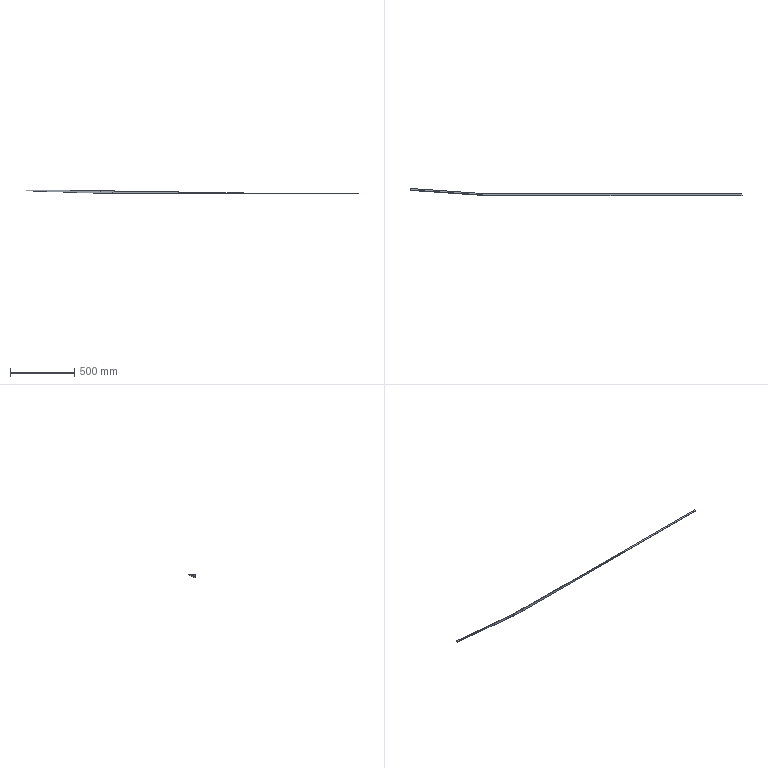Part | SolidWorks | features BaseBody 1 | 1 solid | 18 faces | box 2582 x 55.311 x 25.611 mm | volume 177639 mm3 | plane 18
STEP:
#1=CARTESIAN_POINT('',(2000.,-23.156,0.4292));
#2=VERTEX_POINT('',#1);
#3=CARTESIAN_POINT('',(90.138,-23.157,0.4297));
#4=VERTEX_POINT('',#3);
#5=CARTESIAN_POINT('',(2000.,-23.156,0.4292));
#6=DIRECTION('',(-1.,-0.00000047,0.000000257));
#7=VECTOR('',#6,1000.);
#8=LINE('',#5,#7);
#9=EDGE_CURVE('',#2,#4,#8,.T.);
#10=ORIENTED_EDGE('',*,*,#9,.T.);
#11=CARTESIAN_POINT('',(90.189,-23.22,3.629));
#12=VERTEX_POINT('',#11);
#13=CARTESIAN_POINT('',(90.138,-23.157,0.4297));
#14=DIRECTION('',(0.01588,-0.01967,0.9997));
#15=VECTOR('',#14,1000.);
#16=LINE('',#13,#15);
#17=EDGE_CURVE('',#4,#12,#16,.T.);
#18=ORIENTED_EDGE('',*,*,#17,.T.);
#19=CARTESIAN_POINT('',(2000.,-23.219,3.629));
#20=VERTEX_POINT('',#19);
#21=CARTESIAN_POINT('',(90.189,-23.22,3.629));
#22=DIRECTION('',(1.,0.00000047,-0.000000257));
#23=VECTOR('',#22,1000.);
#24=LINE('',#21,#23);
#25=EDGE_CURVE('',#12,#20,#24,.T.);
#26=ORIENTED_EDGE('',*,*,#25,.T.);
#27=CARTESIAN_POINT('',(2000.,-23.188,2.029));
#28=DIRECTION('',(0.,0.01967,-0.9998));
#29=VECTOR('',#28,1000.);
#30=LINE('',#27,#29);
#31=EDGE_CURVE('',#20,#2,#30,.T.);
#32=ORIENTED_EDGE('',*,*,#31,.T.);
#33=EDGE_LOOP('',(#10,#18,#26,#32));
#34=FACE_OUTER_BOUND('',#33,.T.);
#35=CARTESIAN_POINT('',(78.679,-23.157,0.41));
#36=DIRECTION('',(-0.000000465,0.9998,0.01967));
#37=DIRECTION('',(0.,-0.01967,0.9998));
#38=AXIS2_PLACEMENT_3D('',#35,#36,#37);
#39=PLANE('',#38);
#40=ADVANCED_FACE('',(#34),#39,.T.);
#41=CARTESIAN_POINT('',(-5.976,-23.214,3.483));
#42=VERTEX_POINT('',#41);
#43=CARTESIAN_POINT('',(-5.976,-23.214,3.483));
#44=DIRECTION('',(0.9995,0.0005894,-0.03175));
#45=VECTOR('',#44,1000.);
#46=LINE('',#43,#45);
#47=EDGE_CURVE('',#42,#4,#46,.T.);
#48=ORIENTED_EDGE('',*,*,#47,.F.);
#49=CARTESIAN_POINT('',(-5.875,-23.277,6.68));
#50=VERTEX_POINT('',#49);
#51=CARTESIAN_POINT('',(-5.875,-23.277,6.68));
#52=DIRECTION('',(-0.03175,0.01966,-0.9993));
#53=VECTOR('',#52,1000.);
#54=LINE('',#51,#53);
#55=EDGE_CURVE('',#50,#42,#54,.T.);
#56=ORIENTED_EDGE('',*,*,#55,.F.);
#57=CARTESIAN_POINT('',(90.189,-23.22,3.629));
#58=DIRECTION('',(-0.9995,-0.0005894,0.03175));
#59=VECTOR('',#58,1000.);
#60=LINE('',#57,#59);
#61=EDGE_CURVE('',#12,#50,#60,.T.);
#62=ORIENTED_EDGE('',*,*,#61,.F.);
#63=ORIENTED_EDGE('',*,*,#17,.F.);
#64=EDGE_LOOP('',(#48,#56,#62,#63));
#65=FACE_OUTER_BOUND('',#64,.T.);
#66=CARTESIAN_POINT('',(-6.553,-23.278,6.718));
#67=DIRECTION('',(-0.00003526,-0.9998,-0.01967));
#68=DIRECTION('',(0.,0.01967,-0.9998));
#69=AXIS2_PLACEMENT_3D('',#66,#67,#68);
#70=PLANE('',#69);
#71=ADVANCED_FACE('',(#65),#70,.F.);
#72=CARTESIAN_POINT('',(2000.,-38.156,0.1341));
#73=VERTEX_POINT('',#72);
#74=CARTESIAN_POINT('',(90.138,-38.157,0.1346));
#75=VERTEX_POINT('',#74);
#76=CARTESIAN_POINT('',(2000.,-38.156,0.1341));
#77=DIRECTION('',(-1.,-0.00000047,0.000000257));
#78=VECTOR('',#77,1000.);
#79=LINE('',#76,#78);
#80=EDGE_CURVE('',#73,#75,#79,.T.);
#81=ORIENTED_EDGE('',*,*,#80,.T.);
#82=CARTESIAN_POINT('',(90.138,-38.157,0.1346));
#83=DIRECTION('',(0.00001742,0.9998,0.01967));
#84=VECTOR('',#83,1000.);
#85=LINE('',#82,#84);
#86=EDGE_CURVE('',#75,#4,#85,.T.);
#87=ORIENTED_EDGE('',*,*,#86,.T.);
#88=ORIENTED_EDGE('',*,*,#9,.F.);
#89=CARTESIAN_POINT('',(2000.,-38.247,0.1323));
#90=DIRECTION('',(0.,-0.9998,-0.01967));
#91=VECTOR('',#90,1000.);
#92=LINE('',#89,#91);
#93=EDGE_CURVE('',#2,#73,#92,.T.);
#94=ORIENTED_EDGE('',*,*,#93,.T.);
#95=EDGE_LOOP('',(#81,#87,#88,#94));
#96=FACE_OUTER_BOUND('',#95,.T.);
#97=CARTESIAN_POINT('',(78.679,-38.247,0.1328));
#98=DIRECTION('',(-0.000000266,0.01967,-0.9998));
#99=DIRECTION('',(0.,0.9998,0.01967));
#100=AXIS2_PLACEMENT_3D('',#97,#98,#99);
#101=PLANE('',#100);
#102=ADVANCED_FACE('',(#96),#101,.T.);
#103=ORIENTED_EDGE('',*,*,#93,.F.);
#104=ORIENTED_EDGE('',*,*,#31,.F.);
#105=CARTESIAN_POINT('',(2000.,-38.219,3.333));
#106=VERTEX_POINT('',#105);
#107=CARTESIAN_POINT('',(2000.,-23.219,3.629));
#108=DIRECTION('',(0.000000465,-0.9998,-0.01967));
#109=VECTOR('',#108,1000.);
#110=LINE('',#107,#109);
#111=EDGE_CURVE('',#20,#106,#110,.T.);
#112=ORIENTED_EDGE('',*,*,#111,.T.);
#113=CARTESIAN_POINT('',(2000.,-38.219,3.333));
#114=DIRECTION('',(-0.000000266,0.01967,-0.9998));
#115=VECTOR('',#114,1000.);
#116=LINE('',#113,#115);
#117=EDGE_CURVE('',#106,#73,#116,.T.);
#118=ORIENTED_EDGE('',*,*,#117,.T.);
#119=EDGE_LOOP('',(#103,#104,#112,#118));
#120=FACE_OUTER_BOUND('',#119,.T.);
#121=CARTESIAN_POINT('',(2000.,-38.309,0.1131));
#122=DIRECTION('',(1.,0.00000047,-0.000000257));
#123=DIRECTION('',(-0.00000047,1.,0.));
#124=AXIS2_PLACEMENT_3D('',#121,#122,#123);
#125=PLANE('',#124);
#126=ADVANCED_FACE('',(#120),#125,.T.);
#127=ORIENTED_EDGE('',*,*,#25,.F.);
#128=CARTESIAN_POINT('',(90.189,-35.02,3.397));
#129=VERTEX_POINT('',#128);
#130=CARTESIAN_POINT('',(90.189,-23.22,3.629));
#131=DIRECTION('',(-0.00001748,-0.9998,-0.01967));
#132=VECTOR('',#131,1000.);
#133=LINE('',#130,#132);
#134=EDGE_CURVE('',#12,#129,#133,.T.);
#135=ORIENTED_EDGE('',*,*,#134,.T.);
#136=CARTESIAN_POINT('',(1223.273,-35.02,3.397));
#137=VERTEX_POINT('',#136);
#138=CARTESIAN_POINT('',(90.189,-35.02,3.397));
#139=DIRECTION('',(1.,0.00000047,-0.000000257));
#140=VECTOR('',#139,1000.);
#141=LINE('',#138,#140);
#142=EDGE_CURVE('',#129,#137,#141,.T.);
#143=ORIENTED_EDGE('',*,*,#142,.T.);
#144=CARTESIAN_POINT('',(1223.273,-38.219,3.334));
#145=VERTEX_POINT('',#144);
#146=CARTESIAN_POINT('',(1223.273,-30.719,3.481));
#147=DIRECTION('',(0.,-0.9998,-0.01967));
#148=VECTOR('',#147,1000.);
#149=LINE('',#146,#148);
#150=EDGE_CURVE('',#137,#145,#149,.T.);
#151=ORIENTED_EDGE('',*,*,#150,.T.);
#152=CARTESIAN_POINT('',(1223.273,-38.219,3.334));
#153=DIRECTION('',(1.,0.00000047,-0.000000257));
#154=VECTOR('',#153,1000.);
#155=LINE('',#152,#154);
#156=EDGE_CURVE('',#145,#106,#155,.T.);
#157=ORIENTED_EDGE('',*,*,#156,.T.);
#158=ORIENTED_EDGE('',*,*,#111,.F.);
#159=EDGE_LOOP('',(#127,#135,#143,#151,#157,#158));
#160=FACE_OUTER_BOUND('',#159,.T.);
#161=CARTESIAN_POINT('',(90.189,-23.219,3.629));
#162=DIRECTION('',(0.000000266,-0.01967,0.9998));
#163=DIRECTION('',(0.,-0.9998,-0.01967));
#164=AXIS2_PLACEMENT_3D('',#161,#162,#163);
#165=PLANE('',#164);
#166=ADVANCED_FACE('',(#160),#165,.T.);
#167=CARTESIAN_POINT('',(-6.5,-38.214,3.204));
#168=VERTEX_POINT('',#167);
#169=CARTESIAN_POINT('',(-582.328,1.725,22.286));
#170=VERTEX_POINT('',#169);
#171=CARTESIAN_POINT('',(-6.5,-38.214,3.204));
#172=DIRECTION('',(-0.9971,0.06916,0.03304));
#173=VECTOR('',#172,1000.);
#174=LINE('',#171,#173);
#175=EDGE_CURVE('',#168,#170,#174,.T.);
#176=ORIENTED_EDGE('',*,*,#175,.T.);
#177=CARTESIAN_POINT('',(-581.281,16.689,22.548));
#178=VERTEX_POINT('',#177);
#179=CARTESIAN_POINT('',(-582.328,1.725,22.286));
#180=DIRECTION('',(0.06976,0.9974,0.01741));
#181=VECTOR('',#180,1000.);
#182=LINE('',#179,#181);
#183=EDGE_CURVE('',#170,#178,#182,.T.);
#184=ORIENTED_EDGE('',*,*,#183,.T.);
#185=CARTESIAN_POINT('',(-581.281,16.689,22.548));
#186=DIRECTION('',(0.9971,-0.06916,-0.03304));
#187=VECTOR('',#186,1000.);
#188=LINE('',#185,#187);
#189=EDGE_CURVE('',#178,#42,#188,.T.);
#190=ORIENTED_EDGE('',*,*,#189,.T.);
#191=ORIENTED_EDGE('',*,*,#47,.T.);
#192=ORIENTED_EDGE('',*,*,#86,.F.);
#193=CARTESIAN_POINT('',(90.138,-38.157,0.1346));
#194=DIRECTION('',(-0.9995,-0.0005894,0.03175));
#195=VECTOR('',#194,1000.);
#196=LINE('',#193,#195);
#197=EDGE_CURVE('',#75,#168,#196,.T.);
#198=ORIENTED_EDGE('',*,*,#197,.T.);
#199=EDGE_LOOP('',(#176,#184,#190,#191,#192,#198));
#200=FACE_OUTER_BOUND('',#199,.T.);
#201=CARTESIAN_POINT('',(90.138,-38.214,0.1335));
#202=DIRECTION('',(-0.03175,0.01966,-0.9993));
#203=DIRECTION('',(-0.9995,0.,0.03176));
#204=AXIS2_PLACEMENT_3D('',#201,#202,#203);
#205=PLANE('',#204);
#206=ADVANCED_FACE('',(#200),#205,.T.);
#207=ORIENTED_EDGE('',*,*,#189,.F.);
#208=CARTESIAN_POINT('',(-581.18,16.626,25.745));
#209=VERTEX_POINT('',#208);
#210=CARTESIAN_POINT('',(-581.281,16.689,22.548));
#211=DIRECTION('',(0.03175,-0.01966,0.9993));
#212=VECTOR('',#211,1000.);
#213=LINE('',#210,#212);
#214=EDGE_CURVE('',#178,#209,#213,.T.);
#215=ORIENTED_EDGE('',*,*,#214,.T.);
#216=CARTESIAN_POINT('',(-581.18,16.626,25.745));
#217=DIRECTION('',(0.9971,-0.06916,-0.03304));
#218=VECTOR('',#217,1000.);
#219=LINE('',#216,#218);
#220=EDGE_CURVE('',#209,#50,#219,.T.);
#221=ORIENTED_EDGE('',*,*,#220,.T.);
#222=ORIENTED_EDGE('',*,*,#55,.T.);
#223=EDGE_LOOP('',(#207,#215,#221,#222));
#224=FACE_OUTER_BOUND('',#223,.T.);
#225=CARTESIAN_POINT('',(-2.418,-23.46,3.349));
#226=DIRECTION('',(0.06976,0.9974,0.01741));
#227=DIRECTION('',(-0.9976,0.06977,0.));
#228=AXIS2_PLACEMENT_3D('',#225,#226,#227);
#229=PLANE('',#228);
#230=ADVANCED_FACE('',(#224),#229,.T.);
#231=ORIENTED_EDGE('',*,*,#220,.F.);
#232=CARTESIAN_POINT('',(-582.003,4.854,25.54));
#233=VERTEX_POINT('',#232);
#234=CARTESIAN_POINT('',(-581.18,16.626,25.745));
#235=DIRECTION('',(-0.06976,-0.9974,-0.01741));
#236=VECTOR('',#235,1000.);
#237=LINE('',#234,#236);
#238=EDGE_CURVE('',#209,#233,#237,.T.);
#239=ORIENTED_EDGE('',*,*,#238,.T.);
#240=CARTESIAN_POINT('',(-6.287,-35.077,6.461));
#241=VERTEX_POINT('',#240);
#242=CARTESIAN_POINT('',(-582.003,4.854,25.54));
#243=DIRECTION('',(0.9971,-0.06916,-0.03304));
#244=VECTOR('',#243,1000.);
#245=LINE('',#242,#244);
#246=EDGE_CURVE('',#233,#241,#245,.T.);
#247=ORIENTED_EDGE('',*,*,#246,.T.);
#248=CARTESIAN_POINT('',(-6.287,-35.077,6.461));
#249=DIRECTION('',(0.9995,0.0005894,-0.03175));
#250=VECTOR('',#249,1000.);
#251=LINE('',#248,#250);
#252=EDGE_CURVE('',#241,#129,#251,.T.);
#253=ORIENTED_EDGE('',*,*,#252,.T.);
#254=ORIENTED_EDGE('',*,*,#134,.F.);
#255=ORIENTED_EDGE('',*,*,#61,.T.);
#256=EDGE_LOOP('',(#231,#239,#247,#253,#254,#255));
#257=FACE_OUTER_BOUND('',#256,.T.);
#258=CARTESIAN_POINT('',(-582.028,-35.077,24.755));
#259=DIRECTION('',(0.03175,-0.01966,0.9993));
#260=DIRECTION('',(0.9995,0.,-0.03176));
#261=AXIS2_PLACEMENT_3D('',#258,#259,#260);
#262=PLANE('',#261);
#263=ADVANCED_FACE('',(#257),#262,.T.);
#264=ORIENTED_EDGE('',*,*,#80,.F.);
#265=ORIENTED_EDGE('',*,*,#117,.F.);
#266=ORIENTED_EDGE('',*,*,#156,.F.);
#267=CARTESIAN_POINT('',(90.468,-38.566,20.934));
#268=VERTEX_POINT('',#267);
#269=CARTESIAN_POINT('',(1223.273,-38.219,3.334));
#270=DIRECTION('',(-0.9999,-0.0003061,0.01553));
#271=VECTOR('',#270,1000.);
#272=LINE('',#269,#271);
#273=EDGE_CURVE('',#145,#268,#272,.T.);
#274=ORIENTED_EDGE('',*,*,#273,.T.);
#275=CARTESIAN_POINT('',(90.468,-38.566,20.934));
#276=DIRECTION('',(-0.01588,0.01967,-0.9997));
#277=VECTOR('',#276,1000.);
#278=LINE('',#275,#277);
#279=EDGE_CURVE('',#268,#75,#278,.T.);
#280=ORIENTED_EDGE('',*,*,#279,.T.);
#281=EDGE_LOOP('',(#264,#265,#266,#274,#280));
#282=FACE_OUTER_BOUND('',#281,.T.);
#283=CARTESIAN_POINT('',(90.138,-38.566,20.934));
#284=DIRECTION('',(0.000000465,-0.9998,-0.01967));
#285=DIRECTION('',(0.,0.01967,-0.9998));
#286=AXIS2_PLACEMENT_3D('',#283,#284,#285);
#287=PLANE('',#286);
#288=ADVANCED_FACE('',(#282),#287,.T.);
#289=ORIENTED_EDGE('',*,*,#150,.F.);
#290=CARTESIAN_POINT('',(90.468,-35.367,20.997));
#291=VERTEX_POINT('',#290);
#292=CARTESIAN_POINT('',(90.468,-35.367,20.997));
#293=DIRECTION('',(0.9999,0.0003061,-0.01553));
#294=VECTOR('',#293,1000.);
#295=LINE('',#292,#294);
#296=EDGE_CURVE('',#291,#137,#295,.T.);
#297=ORIENTED_EDGE('',*,*,#296,.F.);
#298=CARTESIAN_POINT('',(90.468,-38.566,20.934));
#299=DIRECTION('',(0.00003449,0.9998,0.01967));
#300=VECTOR('',#299,1000.);
#301=LINE('',#298,#300);
#302=EDGE_CURVE('',#268,#291,#301,.T.);
#303=ORIENTED_EDGE('',*,*,#302,.F.);
#304=ORIENTED_EDGE('',*,*,#273,.F.);
#305=EDGE_LOOP('',(#289,#297,#303,#304));
#306=FACE_OUTER_BOUND('',#305,.T.);
#307=CARTESIAN_POINT('',(90.468,-38.585,20.933));
#308=DIRECTION('',(-0.01554,0.01967,-0.9997));
#309=DIRECTION('',(0.,0.9998,0.01967));
#310=AXIS2_PLACEMENT_3D('',#307,#308,#309);
#311=PLANE('',#310);
#312=ADVANCED_FACE('',(#306),#311,.F.);
#313=ORIENTED_EDGE('',*,*,#142,.F.);
#314=CARTESIAN_POINT('',(90.189,-35.02,3.397));
#315=DIRECTION('',(0.01588,-0.01967,0.9997));
#316=VECTOR('',#315,1000.);
#317=LINE('',#314,#316);
#318=EDGE_CURVE('',#129,#291,#317,.T.);
#319=ORIENTED_EDGE('',*,*,#318,.T.);
#320=ORIENTED_EDGE('',*,*,#296,.T.);
#321=EDGE_LOOP('',(#313,#319,#320));
#322=FACE_OUTER_BOUND('',#321,.T.);
#323=CARTESIAN_POINT('',(83.39,-35.018,3.291));
#324=DIRECTION('',(-0.000000465,0.9998,0.01967));
#325=DIRECTION('',(0.,-0.01967,0.9998));
#326=AXIS2_PLACEMENT_3D('',#323,#324,#325);
#327=PLANE('',#326);
#328=ADVANCED_FACE('',(#322),#327,.T.);
#329=CARTESIAN_POINT('',(-582.226,1.662,25.484));
#330=VERTEX_POINT('',#329);
#331=CARTESIAN_POINT('',(-582.003,4.854,25.54));
#332=DIRECTION('',(-0.06976,-0.9974,-0.01741));
#333=VECTOR('',#332,1000.);
#334=LINE('',#331,#333);
#335=EDGE_CURVE('',#233,#330,#334,.T.);
#336=ORIENTED_EDGE('',*,*,#335,.F.);
#337=ORIENTED_EDGE('',*,*,#238,.F.);
#338=ORIENTED_EDGE('',*,*,#214,.F.);
#339=ORIENTED_EDGE('',*,*,#183,.F.);
#340=CARTESIAN_POINT('',(-582.226,1.662,25.484));
#341=DIRECTION('',(-0.03175,0.01966,-0.9993));
#342=VECTOR('',#341,1000.);
#343=LINE('',#340,#342);
#344=EDGE_CURVE('',#330,#170,#343,.T.);
#345=ORIENTED_EDGE('',*,*,#344,.F.);
#346=EDGE_LOOP('',(#336,#337,#338,#339,#345));
#347=FACE_OUTER_BOUND('',#346,.T.);
#348=CARTESIAN_POINT('',(-582.332,1.67,22.286));
#349=DIRECTION('',(0.9971,-0.06916,-0.03304));
#350=DIRECTION('',(0.06919,0.9976,0.));
#351=AXIS2_PLACEMENT_3D('',#348,#349,#350);
#352=PLANE('',#351);
#353=ADVANCED_FACE('',(#347),#352,.F.);
#354=CARTESIAN_POINT('',(-5.84,-38.623,23.993));
#355=VERTEX_POINT('',#354);
#356=CARTESIAN_POINT('',(-6.5,-38.214,3.204));
#357=DIRECTION('',(0.03175,-0.01966,0.9993));
#358=VECTOR('',#357,1000.);
#359=LINE('',#356,#358);
#360=EDGE_CURVE('',#168,#355,#359,.T.);
#361=ORIENTED_EDGE('',*,*,#360,.T.);
#362=CARTESIAN_POINT('',(-5.951,-38.615,23.996));
#363=VERTEX_POINT('',#362);
#364=CARTESIAN_POINT('',(-5.84,-38.623,23.993));
#365=DIRECTION('',(-0.9971,0.06916,0.03304));
#366=VECTOR('',#365,1000.);
#367=LINE('',#364,#366);
#368=EDGE_CURVE('',#355,#363,#367,.T.);
#369=ORIENTED_EDGE('',*,*,#368,.T.);
#370=CARTESIAN_POINT('',(-5.951,-38.615,23.996));
#371=DIRECTION('',(-0.9976,0.06972,0.002575));
#372=VECTOR('',#371,1000.);
#373=LINE('',#370,#372);
#374=EDGE_CURVE('',#363,#330,#373,.T.);
#375=ORIENTED_EDGE('',*,*,#374,.T.);
#376=ORIENTED_EDGE('',*,*,#344,.T.);
#377=ORIENTED_EDGE('',*,*,#175,.F.);
#378=EDGE_LOOP('',(#361,#369,#375,#376,#377));
#379=FACE_OUTER_BOUND('',#378,.T.);
#380=CARTESIAN_POINT('',(-582.305,2.057,3.204));
#381=DIRECTION('',(-0.06976,-0.9974,-0.01741));
#382=DIRECTION('',(0.9976,-0.06977,0.));
#383=AXIS2_PLACEMENT_3D('',#380,#381,#382);
#384=PLANE('',#383);
#385=ADVANCED_FACE('',(#379),#384,.T.);
#386=CARTESIAN_POINT('',(-5.84,-38.623,23.993));
#387=DIRECTION('',(0.9995,0.0005894,-0.03175));
#388=VECTOR('',#387,1000.);
#389=LINE('',#386,#388);
#390=EDGE_CURVE('',#355,#268,#389,.T.);
#391=ORIENTED_EDGE('',*,*,#390,.F.);
#392=ORIENTED_EDGE('',*,*,#360,.F.);
#393=ORIENTED_EDGE('',*,*,#197,.F.);
#394=ORIENTED_EDGE('',*,*,#279,.F.);
#395=EDGE_LOOP('',(#391,#392,#393,#394));
#396=FACE_OUTER_BOUND('',#395,.T.);
#397=CARTESIAN_POINT('',(-7.082,-38.15,-0.008479));
#398=DIRECTION('',(0.00003526,0.9998,0.01967));
#399=DIRECTION('',(0.,-0.01967,0.9998));
#400=AXIS2_PLACEMENT_3D('',#397,#398,#399);
#401=PLANE('',#400);
#402=ADVANCED_FACE('',(#396),#401,.F.);
#403=ORIENTED_EDGE('',*,*,#252,.F.);
#404=CARTESIAN_POINT('',(-5.728,-35.423,24.052));
#405=VERTEX_POINT('',#404);
#406=CARTESIAN_POINT('',(-5.728,-35.423,24.052));
#407=DIRECTION('',(-0.03175,0.01966,-0.9993));
#408=VECTOR('',#407,1000.);
#409=LINE('',#406,#408);
#410=EDGE_CURVE('',#405,#241,#409,.T.);
#411=ORIENTED_EDGE('',*,*,#410,.F.);
#412=CARTESIAN_POINT('',(90.468,-35.367,20.997));
#413=DIRECTION('',(-0.9995,-0.0005894,0.03175));
#414=VECTOR('',#413,1000.);
#415=LINE('',#412,#414);
#416=EDGE_CURVE('',#291,#405,#415,.T.);
#417=ORIENTED_EDGE('',*,*,#416,.F.);
#418=ORIENTED_EDGE('',*,*,#318,.F.);
#419=EDGE_LOOP('',(#403,#411,#417,#418));
#420=FACE_OUTER_BOUND('',#419,.T.);
#421=CARTESIAN_POINT('',(-6.868,-35.426,24.176));
#422=DIRECTION('',(-0.00003526,-0.9998,-0.01967));
#423=DIRECTION('',(0.,0.01967,-0.9998));
#424=AXIS2_PLACEMENT_3D('',#421,#422,#423);
#425=PLANE('',#424);
#426=ADVANCED_FACE('',(#420),#425,.F.);
#427=ORIENTED_EDGE('',*,*,#410,.T.);
#428=ORIENTED_EDGE('',*,*,#246,.F.);
#429=CARTESIAN_POINT('',(-582.003,4.854,25.54));
#430=DIRECTION('',(0.9976,-0.06972,-0.002575));
#431=VECTOR('',#430,1000.);
#432=LINE('',#429,#431);
#433=EDGE_CURVE('',#233,#405,#432,.T.);
#434=ORIENTED_EDGE('',*,*,#433,.T.);
#435=EDGE_LOOP('',(#427,#428,#434));
#436=FACE_OUTER_BOUND('',#435,.T.);
#437=CARTESIAN_POINT('',(-2.249,-35.358,6.347));
#438=DIRECTION('',(0.06976,0.9974,0.01741));
#439=DIRECTION('',(-0.9976,0.06977,0.));
#440=AXIS2_PLACEMENT_3D('',#437,#438,#439);
#441=PLANE('',#440);
#442=ADVANCED_FACE('',(#436),#441,.T.);
#443=ORIENTED_EDGE('',*,*,#302,.T.);
#444=ORIENTED_EDGE('',*,*,#416,.T.);
#445=CARTESIAN_POINT('',(-5.728,-35.423,24.052));
#446=DIRECTION('',(-0.06976,-0.9974,-0.01741));
#447=VECTOR('',#446,1000.);
#448=LINE('',#445,#447);
#449=EDGE_CURVE('',#405,#363,#448,.T.);
#450=ORIENTED_EDGE('',*,*,#449,.T.);
#451=ORIENTED_EDGE('',*,*,#368,.F.);
#452=ORIENTED_EDGE('',*,*,#390,.T.);
#453=EDGE_LOOP('',(#443,#444,#450,#451,#452));
#454=FACE_OUTER_BOUND('',#453,.T.);
#455=CARTESIAN_POINT('',(-5.951,-38.623,23.996));
#456=DIRECTION('',(0.03175,-0.01966,0.9993));
#457=DIRECTION('',(0.9995,0.,-0.03176));
#458=AXIS2_PLACEMENT_3D('',#455,#456,#457);
#459=PLANE('',#458);
#460=ADVANCED_FACE('',(#454),#459,.T.);
#461=ORIENTED_EDGE('',*,*,#449,.F.);
#462=ORIENTED_EDGE('',*,*,#433,.F.);
#463=ORIENTED_EDGE('',*,*,#335,.T.);
#464=ORIENTED_EDGE('',*,*,#374,.F.);
#465=EDGE_LOOP('',(#461,#462,#463,#464));
#466=FACE_OUTER_BOUND('',#465,.T.);
#467=CARTESIAN_POINT('',(-585.685,-38.89,24.777));
#468=DIRECTION('',(-0.001355,0.01755,-0.9998));
#469=DIRECTION('',(0.,0.9998,0.01755));
#470=AXIS2_PLACEMENT_3D('',#467,#468,#469);
#471=PLANE('',#470);
#472=ADVANCED_FACE('',(#466),#471,.F.);
#473=CLOSED_SHELL('',(#40,#71,#102,#126,#166,#206,#230,#263,#288,#312,#328,#353,#385,#402,#426,#442,#460,#472));
#474=MANIFOLD_SOLID_BREP('',#473);
#475=CARTESIAN_POINT('',(0.,0.,0.));
#476=DIRECTION('',(0.,0.,1.));
#477=DIRECTION('',(1.,0.,0.));
#478=AXIS2_PLACEMENT_3D('',#475,#476,#477);
#479=(LENGTH_UNIT()NAMED_UNIT(*)SI_UNIT(.MILLI.,.METRE.));
#480=UNCERTAINTY_MEASURE_WITH_UNIT(LENGTH_MEASURE(0.00001),#479,'','');
#481=(NAMED_UNIT(*)PLANE_ANGLE_UNIT()SI_UNIT($,.RADIAN.));
#482=(NAMED_UNIT(*)SI_UNIT($,.STERADIAN.)SOLID_ANGLE_UNIT());
#483=(GEOMETRIC_REPRESENTATION_CONTEXT(3)GLOBAL_UNCERTAINTY_ASSIGNED_CONTEXT((#480))GLOBAL_UNIT_ASSIGNED_CONTEXT((#479,#481,#482))REPRESENTATION_CONTEXT('',''));
#484=ADVANCED_BREP_SHAPE_REPRESENTATION('',(#474,#478),#483);